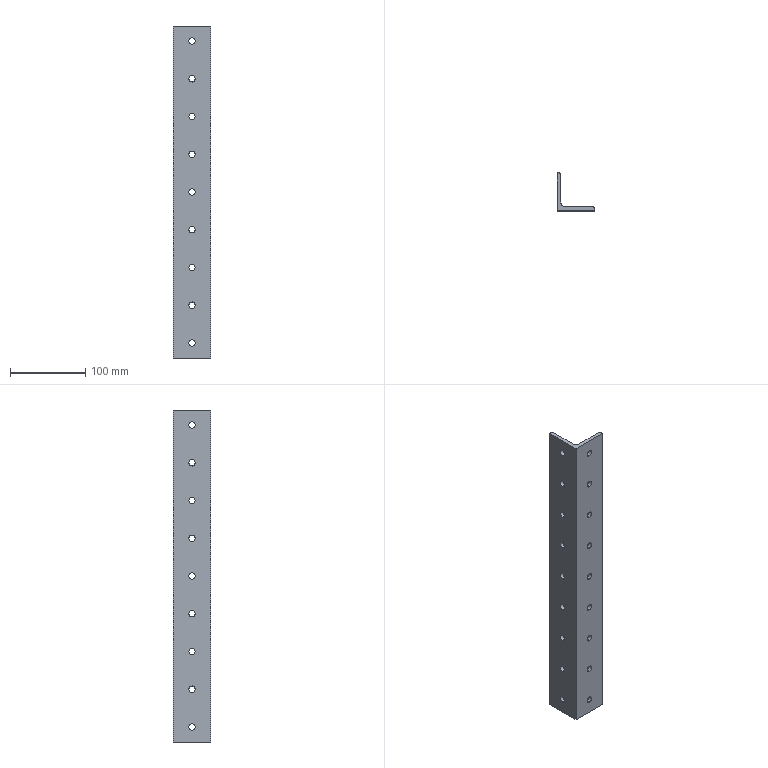Part | STEP file | 750038241 | 1 solid | 47 faces | box 50 x 50 x 440 mm | volume 204554 mm3 | cylinder 39 | plane 8 | commonest cylinder face diameters 8.5 x36 6 x2 10 x1